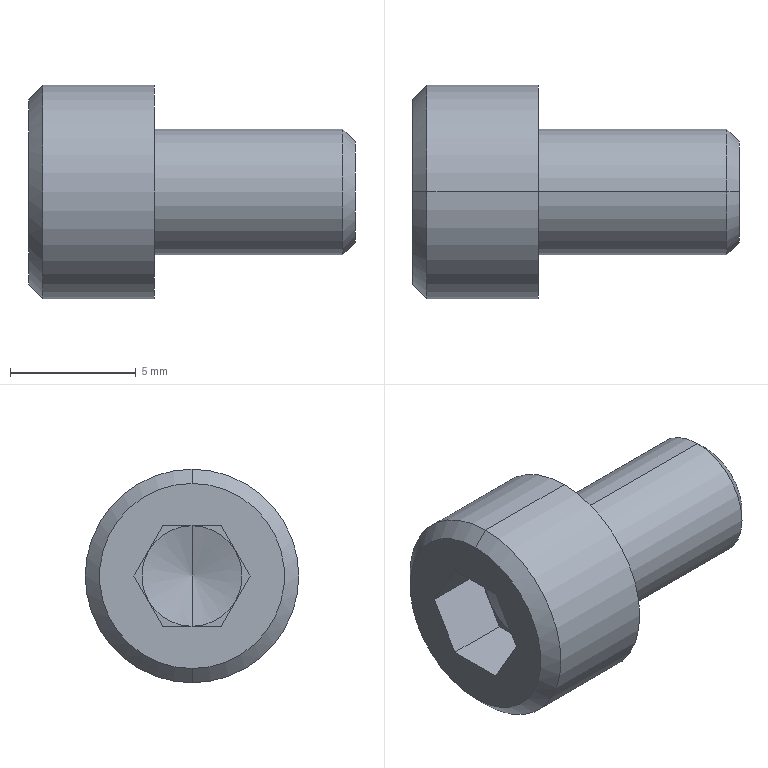Part | STEP file | CB5-8_Default | 1 solid | 25 faces | box 13 x 8.5 x 8.5 mm | volume 398.056 mm3 | plane 15 | cone 6 | cylinder 4 | commonest cylinder face diameters 5 x2 8.5 x2